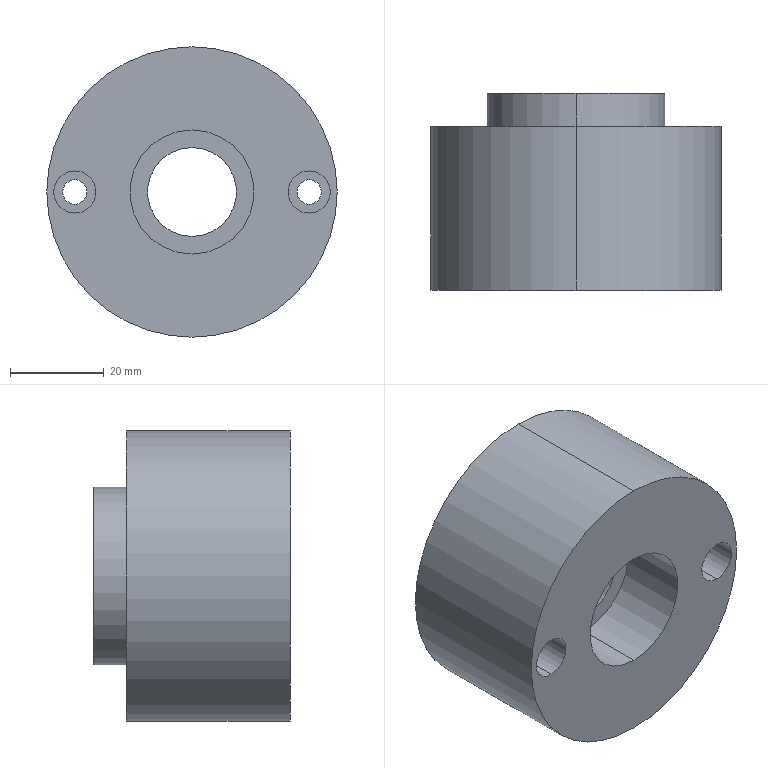Part | 1 solid | 24 faces | box 62 x 42 x 62 mm | volume 87250 mm3 | cylinder 16 | plane 6 | cone 2 | commonest cylinder face diameters 5.2 x4 9 x4 19 x2 26.5 x2 38 x2 62 x2
STEP:
#1=CARTESIAN_POINT('',(0.,20.,9.5));
#2=VERTEX_POINT('',#1);
#3=CARTESIAN_POINT('',(0.,20.,-9.5));
#4=VERTEX_POINT('',#3);
#5=CARTESIAN_POINT('',(0.,20.,0.));
#6=DIRECTION('',(0.,-1.,0.));
#7=DIRECTION('',(0.,0.,-1.));
#8=AXIS2_PLACEMENT_3D('',#5,#6,#7);
#9=CIRCLE('',#8,9.5);
#10=EDGE_CURVE('',#2,#4,#9,.T.);
#11=ORIENTED_EDGE('',*,*,#10,.T.);
#12=CARTESIAN_POINT('',(0.,42.,-18.));
#13=VERTEX_POINT('',#12);
#14=CARTESIAN_POINT('',(0.,20.,-9.5));
#15=DIRECTION('',(0.,0.9328,-0.3604));
#16=VECTOR('',#15,1000.);
#17=LINE('',#14,#16);
#18=EDGE_CURVE('',#4,#13,#17,.T.);
#19=ORIENTED_EDGE('',*,*,#18,.T.);
#20=CARTESIAN_POINT('',(0.,42.,18.));
#21=VERTEX_POINT('',#20);
#22=CARTESIAN_POINT('',(0.,42.,0.));
#23=DIRECTION('',(0.,-1.,0.));
#24=DIRECTION('',(0.,0.,-1.));
#25=AXIS2_PLACEMENT_3D('',#22,#23,#24);
#26=CIRCLE('',#25,18.);
#27=EDGE_CURVE('',#21,#13,#26,.T.);
#28=ORIENTED_EDGE('',*,*,#27,.F.);
#29=CARTESIAN_POINT('',(0.,20.,9.5));
#30=DIRECTION('',(0.,0.9328,0.3604));
#31=VECTOR('',#30,1000.);
#32=LINE('',#29,#31);
#33=EDGE_CURVE('',#2,#21,#32,.T.);
#34=ORIENTED_EDGE('',*,*,#33,.F.);
#35=EDGE_LOOP('',(#11,#19,#28,#34));
#36=FACE_OUTER_BOUND('',#35,.T.);
#37=CARTESIAN_POINT('',(0.,20.,0.));
#38=DIRECTION('',(0.,1.,0.));
#39=DIRECTION('',(0.,0.,1.));
#40=AXIS2_PLACEMENT_3D('',#37,#38,#39);
#41=CONICAL_SURFACE('',#40,9.5,0.3687);
#42=ADVANCED_FACE('',(#36),#41,.F.);
#43=ORIENTED_EDGE('',*,*,#10,.F.);
#44=CARTESIAN_POINT('',(0.,15.,9.5));
#45=VERTEX_POINT('',#44);
#46=CARTESIAN_POINT('',(0.,15.,9.5));
#47=DIRECTION('',(0.,-1.,0.));
#48=VECTOR('',#47,1000.);
#49=LINE('',#46,#48);
#50=EDGE_CURVE('',#2,#45,#49,.T.);
#51=ORIENTED_EDGE('',*,*,#50,.T.);
#52=CARTESIAN_POINT('',(0.,15.,-9.5));
#53=VERTEX_POINT('',#52);
#54=CARTESIAN_POINT('',(0.,15.,0.));
#55=DIRECTION('',(0.,-1.,0.));
#56=DIRECTION('',(0.,0.,-1.));
#57=AXIS2_PLACEMENT_3D('',#54,#55,#56);
#58=CIRCLE('',#57,9.5);
#59=EDGE_CURVE('',#45,#53,#58,.T.);
#60=ORIENTED_EDGE('',*,*,#59,.T.);
#61=CARTESIAN_POINT('',(0.,15.,-9.5));
#62=DIRECTION('',(0.,-1.,0.));
#63=VECTOR('',#62,1000.);
#64=LINE('',#61,#63);
#65=EDGE_CURVE('',#4,#53,#64,.T.);
#66=ORIENTED_EDGE('',*,*,#65,.F.);
#67=EDGE_LOOP('',(#43,#51,#60,#66));
#68=FACE_OUTER_BOUND('',#67,.T.);
#69=CARTESIAN_POINT('',(0.,15.,0.));
#70=DIRECTION('',(0.,-1.,0.));
#71=DIRECTION('',(0.,0.,-1.));
#72=AXIS2_PLACEMENT_3D('',#69,#70,#71);
#73=CYLINDRICAL_SURFACE('',#72,9.5);
#74=ADVANCED_FACE('',(#68),#73,.F.);
#75=CARTESIAN_POINT('',(0.,15.,13.25));
#76=VERTEX_POINT('',#75);
#77=CARTESIAN_POINT('',(0.,15.,-13.25));
#78=VERTEX_POINT('',#77);
#79=CARTESIAN_POINT('',(0.,15.,0.));
#80=DIRECTION('',(0.,-1.,0.));
#81=DIRECTION('',(0.,0.,-1.));
#82=AXIS2_PLACEMENT_3D('',#79,#80,#81);
#83=CIRCLE('',#82,13.25);
#84=EDGE_CURVE('',#76,#78,#83,.T.);
#85=ORIENTED_EDGE('',*,*,#84,.F.);
#86=CARTESIAN_POINT('',(0.,0.,13.25));
#87=VERTEX_POINT('',#86);
#88=CARTESIAN_POINT('',(0.,0.,13.25));
#89=DIRECTION('',(0.,-1.,0.));
#90=VECTOR('',#89,1000.);
#91=LINE('',#88,#90);
#92=EDGE_CURVE('',#76,#87,#91,.T.);
#93=ORIENTED_EDGE('',*,*,#92,.T.);
#94=CARTESIAN_POINT('',(0.,0.,-13.25));
#95=VERTEX_POINT('',#94);
#96=CARTESIAN_POINT('',(0.,0.,0.));
#97=DIRECTION('',(0.,-1.,0.));
#98=DIRECTION('',(0.,0.,-1.));
#99=AXIS2_PLACEMENT_3D('',#96,#97,#98);
#100=CIRCLE('',#99,13.25);
#101=EDGE_CURVE('',#87,#95,#100,.T.);
#102=ORIENTED_EDGE('',*,*,#101,.T.);
#103=CARTESIAN_POINT('',(0.,0.,-13.25));
#104=DIRECTION('',(0.,-1.,0.));
#105=VECTOR('',#104,1000.);
#106=LINE('',#103,#105);
#107=EDGE_CURVE('',#78,#95,#106,.T.);
#108=ORIENTED_EDGE('',*,*,#107,.F.);
#109=EDGE_LOOP('',(#85,#93,#102,#108));
#110=FACE_OUTER_BOUND('',#109,.T.);
#111=CARTESIAN_POINT('',(0.,0.,0.));
#112=DIRECTION('',(0.,-1.,0.));
#113=DIRECTION('',(0.,0.,-1.));
#114=AXIS2_PLACEMENT_3D('',#111,#112,#113);
#115=CYLINDRICAL_SURFACE('',#114,13.25);
#116=ADVANCED_FACE('',(#110),#115,.F.);
#117=CARTESIAN_POINT('',(-25.,35.,-2.6));
#118=VERTEX_POINT('',#117);
#119=CARTESIAN_POINT('',(-25.,35.,2.6));
#120=VERTEX_POINT('',#119);
#121=CARTESIAN_POINT('',(-25.,35.,0.));
#122=DIRECTION('',(0.,1.,0.));
#123=DIRECTION('',(0.,0.,1.));
#124=AXIS2_PLACEMENT_3D('',#121,#122,#123);
#125=CIRCLE('',#124,2.6);
#126=EDGE_CURVE('',#118,#120,#125,.T.);
#127=ORIENTED_EDGE('',*,*,#126,.T.);
#128=CARTESIAN_POINT('',(-25.,20.,2.6));
#129=VERTEX_POINT('',#128);
#130=CARTESIAN_POINT('',(-25.,42.,2.6));
#131=DIRECTION('',(0.,-1.,0.));
#132=VECTOR('',#131,1000.);
#133=LINE('',#130,#132);
#134=EDGE_CURVE('',#120,#129,#133,.T.);
#135=ORIENTED_EDGE('',*,*,#134,.T.);
#136=CARTESIAN_POINT('',(-25.,20.,-2.6));
#137=VERTEX_POINT('',#136);
#138=CARTESIAN_POINT('',(-25.,20.,0.));
#139=DIRECTION('',(0.,-1.,0.));
#140=DIRECTION('',(0.,0.,-1.));
#141=AXIS2_PLACEMENT_3D('',#138,#139,#140);
#142=CIRCLE('',#141,2.6);
#143=EDGE_CURVE('',#129,#137,#142,.T.);
#144=ORIENTED_EDGE('',*,*,#143,.T.);
#145=CARTESIAN_POINT('',(-25.,42.,-2.6));
#146=DIRECTION('',(0.,-1.,0.));
#147=VECTOR('',#146,1000.);
#148=LINE('',#145,#147);
#149=EDGE_CURVE('',#118,#137,#148,.T.);
#150=ORIENTED_EDGE('',*,*,#149,.F.);
#151=EDGE_LOOP('',(#127,#135,#144,#150));
#152=FACE_OUTER_BOUND('',#151,.T.);
#153=CARTESIAN_POINT('',(-25.,42.,0.));
#154=DIRECTION('',(0.,-1.,0.));
#155=DIRECTION('',(0.,0.,-1.));
#156=AXIS2_PLACEMENT_3D('',#153,#154,#155);
#157=CYLINDRICAL_SURFACE('',#156,2.6);
#158=ADVANCED_FACE('',(#152),#157,.F.);
#159=CARTESIAN_POINT('',(25.,35.,-2.6));
#160=VERTEX_POINT('',#159);
#161=CARTESIAN_POINT('',(25.,35.,2.6));
#162=VERTEX_POINT('',#161);
#163=CARTESIAN_POINT('',(25.,35.,0.));
#164=DIRECTION('',(0.,1.,0.));
#165=DIRECTION('',(0.,0.,1.));
#166=AXIS2_PLACEMENT_3D('',#163,#164,#165);
#167=CIRCLE('',#166,2.6);
#168=EDGE_CURVE('',#160,#162,#167,.T.);
#169=ORIENTED_EDGE('',*,*,#168,.T.);
#170=CARTESIAN_POINT('',(25.,20.,2.6));
#171=VERTEX_POINT('',#170);
#172=CARTESIAN_POINT('',(25.,42.,2.6));
#173=DIRECTION('',(0.,-1.,0.));
#174=VECTOR('',#173,1000.);
#175=LINE('',#172,#174);
#176=EDGE_CURVE('',#162,#171,#175,.T.);
#177=ORIENTED_EDGE('',*,*,#176,.T.);
#178=CARTESIAN_POINT('',(25.,20.,-2.6));
#179=VERTEX_POINT('',#178);
#180=CARTESIAN_POINT('',(25.,20.,0.));
#181=DIRECTION('',(0.,-1.,0.));
#182=DIRECTION('',(0.,0.,1.));
#183=AXIS2_PLACEMENT_3D('',#180,#181,#182);
#184=CIRCLE('',#183,2.6);
#185=EDGE_CURVE('',#171,#179,#184,.T.);
#186=ORIENTED_EDGE('',*,*,#185,.T.);
#187=CARTESIAN_POINT('',(25.,42.,-2.6));
#188=DIRECTION('',(0.,-1.,0.));
#189=VECTOR('',#188,1000.);
#190=LINE('',#187,#189);
#191=EDGE_CURVE('',#160,#179,#190,.T.);
#192=ORIENTED_EDGE('',*,*,#191,.F.);
#193=EDGE_LOOP('',(#169,#177,#186,#192));
#194=FACE_OUTER_BOUND('',#193,.T.);
#195=CARTESIAN_POINT('',(25.,42.,0.));
#196=DIRECTION('',(0.,-1.,0.));
#197=DIRECTION('',(0.,0.,-1.));
#198=AXIS2_PLACEMENT_3D('',#195,#196,#197);
#199=CYLINDRICAL_SURFACE('',#198,2.6);
#200=ADVANCED_FACE('',(#194),#199,.F.);
#201=CARTESIAN_POINT('',(-25.,20.,4.5));
#202=VERTEX_POINT('',#201);
#203=CARTESIAN_POINT('',(-25.,20.,-4.5));
#204=VERTEX_POINT('',#203);
#205=CARTESIAN_POINT('',(-25.,20.,0.));
#206=DIRECTION('',(0.,-1.,0.));
#207=DIRECTION('',(0.,0.,-1.));
#208=AXIS2_PLACEMENT_3D('',#205,#206,#207);
#209=CIRCLE('',#208,4.5);
#210=EDGE_CURVE('',#202,#204,#209,.T.);
#211=ORIENTED_EDGE('',*,*,#210,.F.);
#212=CARTESIAN_POINT('',(-25.,0.,4.5));
#213=VERTEX_POINT('',#212);
#214=CARTESIAN_POINT('',(-25.,20.,4.5));
#215=DIRECTION('',(0.,-1.,0.));
#216=VECTOR('',#215,1000.);
#217=LINE('',#214,#216);
#218=EDGE_CURVE('',#202,#213,#217,.T.);
#219=ORIENTED_EDGE('',*,*,#218,.T.);
#220=CARTESIAN_POINT('',(-25.,0.,-4.5));
#221=VERTEX_POINT('',#220);
#222=CARTESIAN_POINT('',(-25.,0.,0.));
#223=DIRECTION('',(0.,-1.,0.));
#224=DIRECTION('',(0.,0.,-1.));
#225=AXIS2_PLACEMENT_3D('',#222,#223,#224);
#226=CIRCLE('',#225,4.5);
#227=EDGE_CURVE('',#213,#221,#226,.T.);
#228=ORIENTED_EDGE('',*,*,#227,.T.);
#229=CARTESIAN_POINT('',(-25.,20.,-4.5));
#230=DIRECTION('',(0.,-1.,0.));
#231=VECTOR('',#230,1000.);
#232=LINE('',#229,#231);
#233=EDGE_CURVE('',#204,#221,#232,.T.);
#234=ORIENTED_EDGE('',*,*,#233,.F.);
#235=EDGE_LOOP('',(#211,#219,#228,#234));
#236=FACE_OUTER_BOUND('',#235,.T.);
#237=CARTESIAN_POINT('',(-25.,20.,0.));
#238=DIRECTION('',(0.,-1.,0.));
#239=DIRECTION('',(0.,0.,-1.));
#240=AXIS2_PLACEMENT_3D('',#237,#238,#239);
#241=CYLINDRICAL_SURFACE('',#240,4.5);
#242=ADVANCED_FACE('',(#236),#241,.F.);
#243=CARTESIAN_POINT('',(25.,20.,4.5));
#244=VERTEX_POINT('',#243);
#245=CARTESIAN_POINT('',(25.,20.,-4.5));
#246=VERTEX_POINT('',#245);
#247=CARTESIAN_POINT('',(25.,20.,0.));
#248=DIRECTION('',(0.,-1.,0.));
#249=DIRECTION('',(0.,0.,1.));
#250=AXIS2_PLACEMENT_3D('',#247,#248,#249);
#251=CIRCLE('',#250,4.5);
#252=EDGE_CURVE('',#244,#246,#251,.T.);
#253=ORIENTED_EDGE('',*,*,#252,.F.);
#254=CARTESIAN_POINT('',(25.,0.,4.5));
#255=VERTEX_POINT('',#254);
#256=CARTESIAN_POINT('',(25.,20.,4.5));
#257=DIRECTION('',(0.,-1.,0.));
#258=VECTOR('',#257,1000.);
#259=LINE('',#256,#258);
#260=EDGE_CURVE('',#244,#255,#259,.T.);
#261=ORIENTED_EDGE('',*,*,#260,.T.);
#262=CARTESIAN_POINT('',(25.,0.,-4.5));
#263=VERTEX_POINT('',#262);
#264=CARTESIAN_POINT('',(25.,0.,0.));
#265=DIRECTION('',(0.,-1.,0.));
#266=DIRECTION('',(0.,0.,1.));
#267=AXIS2_PLACEMENT_3D('',#264,#265,#266);
#268=CIRCLE('',#267,4.5);
#269=EDGE_CURVE('',#255,#263,#268,.T.);
#270=ORIENTED_EDGE('',*,*,#269,.T.);
#271=CARTESIAN_POINT('',(25.,20.,-4.5));
#272=DIRECTION('',(0.,-1.,0.));
#273=VECTOR('',#272,1000.);
#274=LINE('',#271,#273);
#275=EDGE_CURVE('',#246,#263,#274,.T.);
#276=ORIENTED_EDGE('',*,*,#275,.F.);
#277=EDGE_LOOP('',(#253,#261,#270,#276));
#278=FACE_OUTER_BOUND('',#277,.T.);
#279=CARTESIAN_POINT('',(25.,20.,0.));
#280=DIRECTION('',(0.,-1.,0.));
#281=DIRECTION('',(0.,0.,-1.));
#282=AXIS2_PLACEMENT_3D('',#279,#280,#281);
#283=CYLINDRICAL_SURFACE('',#282,4.5);
#284=ADVANCED_FACE('',(#278),#283,.F.);
#285=CARTESIAN_POINT('',(0.,42.,19.));
#286=VERTEX_POINT('',#285);
#287=CARTESIAN_POINT('',(0.,42.,-19.));
#288=VERTEX_POINT('',#287);
#289=CARTESIAN_POINT('',(0.,42.,0.));
#290=DIRECTION('',(0.,1.,0.));
#291=DIRECTION('',(0.,0.,1.));
#292=AXIS2_PLACEMENT_3D('',#289,#290,#291);
#293=CIRCLE('',#292,19.);
#294=EDGE_CURVE('',#286,#288,#293,.T.);
#295=ORIENTED_EDGE('',*,*,#294,.F.);
#296=CARTESIAN_POINT('',(0.,35.,19.));
#297=VERTEX_POINT('',#296);
#298=CARTESIAN_POINT('',(0.,42.,19.));
#299=DIRECTION('',(0.,-1.,0.));
#300=VECTOR('',#299,1000.);
#301=LINE('',#298,#300);
#302=EDGE_CURVE('',#286,#297,#301,.T.);
#303=ORIENTED_EDGE('',*,*,#302,.T.);
#304=CARTESIAN_POINT('',(0.,35.,-19.));
#305=VERTEX_POINT('',#304);
#306=CARTESIAN_POINT('',(0.,35.,0.));
#307=DIRECTION('',(0.,1.,0.));
#308=DIRECTION('',(0.,0.,1.));
#309=AXIS2_PLACEMENT_3D('',#306,#307,#308);
#310=CIRCLE('',#309,19.);
#311=EDGE_CURVE('',#297,#305,#310,.T.);
#312=ORIENTED_EDGE('',*,*,#311,.T.);
#313=CARTESIAN_POINT('',(0.,42.,-19.));
#314=DIRECTION('',(0.,-1.,0.));
#315=VECTOR('',#314,1000.);
#316=LINE('',#313,#315);
#317=EDGE_CURVE('',#288,#305,#316,.T.);
#318=ORIENTED_EDGE('',*,*,#317,.F.);
#319=EDGE_LOOP('',(#295,#303,#312,#318));
#320=FACE_OUTER_BOUND('',#319,.T.);
#321=CARTESIAN_POINT('',(0.,42.,0.));
#322=DIRECTION('',(0.,-1.,0.));
#323=DIRECTION('',(0.,0.,-1.));
#324=AXIS2_PLACEMENT_3D('',#321,#322,#323);
#325=CYLINDRICAL_SURFACE('',#324,19.);
#326=ADVANCED_FACE('',(#320),#325,.T.);
#327=CARTESIAN_POINT('',(0.,35.,31.));
#328=VERTEX_POINT('',#327);
#329=CARTESIAN_POINT('',(0.,35.,-31.));
#330=VERTEX_POINT('',#329);
#331=CARTESIAN_POINT('',(0.,35.,0.));
#332=DIRECTION('',(0.,1.,0.));
#333=DIRECTION('',(0.,0.,1.));
#334=AXIS2_PLACEMENT_3D('',#331,#332,#333);
#335=CIRCLE('',#334,31.);
#336=EDGE_CURVE('',#328,#330,#335,.T.);
#337=ORIENTED_EDGE('',*,*,#336,.F.);
#338=CARTESIAN_POINT('',(0.,0.,31.));
#339=VERTEX_POINT('',#338);
#340=CARTESIAN_POINT('',(0.,35.,31.));
#341=DIRECTION('',(0.,-1.,0.));
#342=VECTOR('',#341,1000.);
#343=LINE('',#340,#342);
#344=EDGE_CURVE('',#328,#339,#343,.T.);
#345=ORIENTED_EDGE('',*,*,#344,.T.);
#346=CARTESIAN_POINT('',(0.,0.,-31.));
#347=VERTEX_POINT('',#346);
#348=CARTESIAN_POINT('',(0.,0.,0.));
#349=DIRECTION('',(0.,1.,0.));
#350=DIRECTION('',(0.,0.,1.));
#351=AXIS2_PLACEMENT_3D('',#348,#349,#350);
#352=CIRCLE('',#351,31.);
#353=EDGE_CURVE('',#339,#347,#352,.T.);
#354=ORIENTED_EDGE('',*,*,#353,.T.);
#355=CARTESIAN_POINT('',(0.,35.,-31.));
#356=DIRECTION('',(0.,-1.,0.));
#357=VECTOR('',#356,1000.);
#358=LINE('',#355,#357);
#359=EDGE_CURVE('',#330,#347,#358,.T.);
#360=ORIENTED_EDGE('',*,*,#359,.F.);
#361=EDGE_LOOP('',(#337,#345,#354,#360));
#362=FACE_OUTER_BOUND('',#361,.T.);
#363=CARTESIAN_POINT('',(0.,35.,0.));
#364=DIRECTION('',(0.,-1.,0.));
#365=DIRECTION('',(0.,0.,-1.));
#366=AXIS2_PLACEMENT_3D('',#363,#364,#365);
#367=CYLINDRICAL_SURFACE('',#366,31.);
#368=ADVANCED_FACE('',(#362),#367,.T.);
#369=ORIENTED_EDGE('',*,*,#344,.F.);
#370=CARTESIAN_POINT('',(0.,35.,0.));
#371=DIRECTION('',(0.,1.,0.));
#372=DIRECTION('',(0.,0.,1.));
#373=AXIS2_PLACEMENT_3D('',#370,#371,#372);
#374=CIRCLE('',#373,31.);
#375=EDGE_CURVE('',#330,#328,#374,.T.);
#376=ORIENTED_EDGE('',*,*,#375,.F.);
#377=ORIENTED_EDGE('',*,*,#359,.T.);
#378=CARTESIAN_POINT('',(0.,0.,0.));
#379=DIRECTION('',(0.,1.,0.));
#380=DIRECTION('',(0.,0.,1.));
#381=AXIS2_PLACEMENT_3D('',#378,#379,#380);
#382=CIRCLE('',#381,31.);
#383=EDGE_CURVE('',#347,#339,#382,.T.);
#384=ORIENTED_EDGE('',*,*,#383,.T.);
#385=EDGE_LOOP('',(#369,#376,#377,#384));
#386=FACE_OUTER_BOUND('',#385,.T.);
#387=CARTESIAN_POINT('',(0.,35.,0.));
#388=DIRECTION('',(0.,-1.,0.));
#389=DIRECTION('',(0.,0.,-1.));
#390=AXIS2_PLACEMENT_3D('',#387,#388,#389);
#391=CYLINDRICAL_SURFACE('',#390,31.);
#392=ADVANCED_FACE('',(#386),#391,.T.);
#393=ORIENTED_EDGE('',*,*,#126,.F.);
#394=CARTESIAN_POINT('',(-25.,35.,0.));
#395=DIRECTION('',(0.,1.,0.));
#396=DIRECTION('',(0.,0.,1.));
#397=AXIS2_PLACEMENT_3D('',#394,#395,#396);
#398=CIRCLE('',#397,2.6);
#399=EDGE_CURVE('',#120,#118,#398,.T.);
#400=ORIENTED_EDGE('',*,*,#399,.F.);
#401=EDGE_LOOP('',(#393,#400));
#402=FACE_BOUND('',#401,.T.);
#403=ORIENTED_EDGE('',*,*,#168,.F.);
#404=CARTESIAN_POINT('',(25.,35.,0.));
#405=DIRECTION('',(0.,1.,0.));
#406=DIRECTION('',(0.,0.,1.));
#407=AXIS2_PLACEMENT_3D('',#404,#405,#406);
#408=CIRCLE('',#407,2.6);
#409=EDGE_CURVE('',#162,#160,#408,.T.);
#410=ORIENTED_EDGE('',*,*,#409,.F.);
#411=EDGE_LOOP('',(#403,#410));
#412=FACE_BOUND('',#411,.T.);
#413=CARTESIAN_POINT('',(0.,35.,0.));
#414=DIRECTION('',(0.,1.,0.));
#415=DIRECTION('',(0.,0.,1.));
#416=AXIS2_PLACEMENT_3D('',#413,#414,#415);
#417=CIRCLE('',#416,19.);
#418=EDGE_CURVE('',#305,#297,#417,.T.);
#419=ORIENTED_EDGE('',*,*,#418,.F.);
#420=ORIENTED_EDGE('',*,*,#311,.F.);
#421=EDGE_LOOP('',(#419,#420));
#422=FACE_BOUND('',#421,.T.);
#423=ORIENTED_EDGE('',*,*,#375,.T.);
#424=ORIENTED_EDGE('',*,*,#336,.T.);
#425=EDGE_LOOP('',(#423,#424));
#426=FACE_OUTER_BOUND('',#425,.T.);
#427=CARTESIAN_POINT('',(0.,35.,0.));
#428=DIRECTION('',(0.,1.,0.));
#429=DIRECTION('',(0.,0.,1.));
#430=AXIS2_PLACEMENT_3D('',#427,#428,#429);
#431=PLANE('',#430);
#432=ADVANCED_FACE('',(#402,#412,#422,#426),#431,.T.);
#433=CARTESIAN_POINT('',(0.,0.,0.));
#434=DIRECTION('',(0.,-1.,0.));
#435=DIRECTION('',(0.,0.,-1.));
#436=AXIS2_PLACEMENT_3D('',#433,#434,#435);
#437=CIRCLE('',#436,13.25);
#438=EDGE_CURVE('',#95,#87,#437,.T.);
#439=ORIENTED_EDGE('',*,*,#438,.F.);
#440=ORIENTED_EDGE('',*,*,#101,.F.);
#441=EDGE_LOOP('',(#439,#440));
#442=FACE_BOUND('',#441,.T.);
#443=CARTESIAN_POINT('',(-25.,0.,0.));
#444=DIRECTION('',(0.,-1.,0.));
#445=DIRECTION('',(0.,0.,-1.));
#446=AXIS2_PLACEMENT_3D('',#443,#444,#445);
#447=CIRCLE('',#446,4.5);
#448=EDGE_CURVE('',#221,#213,#447,.T.);
#449=ORIENTED_EDGE('',*,*,#448,.F.);
#450=ORIENTED_EDGE('',*,*,#227,.F.);
#451=EDGE_LOOP('',(#449,#450));
#452=FACE_BOUND('',#451,.T.);
#453=CARTESIAN_POINT('',(25.,0.,0.));
#454=DIRECTION('',(0.,-1.,0.));
#455=DIRECTION('',(0.,0.,1.));
#456=AXIS2_PLACEMENT_3D('',#453,#454,#455);
#457=CIRCLE('',#456,4.5);
#458=EDGE_CURVE('',#263,#255,#457,.T.);
#459=ORIENTED_EDGE('',*,*,#458,.F.);
#460=ORIENTED_EDGE('',*,*,#269,.F.);
#461=EDGE_LOOP('',(#459,#460));
#462=FACE_BOUND('',#461,.T.);
#463=ORIENTED_EDGE('',*,*,#383,.F.);
#464=ORIENTED_EDGE('',*,*,#353,.F.);
#465=EDGE_LOOP('',(#463,#464));
#466=FACE_OUTER_BOUND('',#465,.T.);
#467=CARTESIAN_POINT('',(0.,0.,0.));
#468=DIRECTION('',(0.,1.,0.));
#469=DIRECTION('',(0.,0.,1.));
#470=AXIS2_PLACEMENT_3D('',#467,#468,#469);
#471=PLANE('',#470);
#472=ADVANCED_FACE('',(#442,#452,#462,#466),#471,.F.);
#473=ORIENTED_EDGE('',*,*,#302,.F.);
#474=CARTESIAN_POINT('',(0.,42.,0.));
#475=DIRECTION('',(0.,1.,0.));
#476=DIRECTION('',(0.,0.,1.));
#477=AXIS2_PLACEMENT_3D('',#474,#475,#476);
#478=CIRCLE('',#477,19.);
#479=EDGE_CURVE('',#288,#286,#478,.T.);
#480=ORIENTED_EDGE('',*,*,#479,.F.);
#481=ORIENTED_EDGE('',*,*,#317,.T.);
#482=ORIENTED_EDGE('',*,*,#418,.T.);
#483=EDGE_LOOP('',(#473,#480,#481,#482));
#484=FACE_OUTER_BOUND('',#483,.T.);
#485=CARTESIAN_POINT('',(0.,42.,0.));
#486=DIRECTION('',(0.,-1.,0.));
#487=DIRECTION('',(0.,0.,-1.));
#488=AXIS2_PLACEMENT_3D('',#485,#486,#487);
#489=CYLINDRICAL_SURFACE('',#488,19.);
#490=ADVANCED_FACE('',(#484),#489,.T.);
#491=ORIENTED_EDGE('',*,*,#27,.T.);
#492=CARTESIAN_POINT('',(0.,42.,0.));
#493=DIRECTION('',(0.,-1.,0.));
#494=DIRECTION('',(0.,0.,-1.));
#495=AXIS2_PLACEMENT_3D('',#492,#493,#494);
#496=CIRCLE('',#495,18.);
#497=EDGE_CURVE('',#13,#21,#496,.T.);
#498=ORIENTED_EDGE('',*,*,#497,.T.);
#499=EDGE_LOOP('',(#491,#498));
#500=FACE_BOUND('',#499,.T.);
#501=ORIENTED_EDGE('',*,*,#479,.T.);
#502=ORIENTED_EDGE('',*,*,#294,.T.);
#503=EDGE_LOOP('',(#501,#502));
#504=FACE_OUTER_BOUND('',#503,.T.);
#505=CARTESIAN_POINT('',(0.,42.,0.));
#506=DIRECTION('',(0.,1.,0.));
#507=DIRECTION('',(0.,0.,1.));
#508=AXIS2_PLACEMENT_3D('',#505,#506,#507);
#509=PLANE('',#508);
#510=ADVANCED_FACE('',(#500,#504),#509,.T.);
#511=ORIENTED_EDGE('',*,*,#260,.F.);
#512=CARTESIAN_POINT('',(25.,20.,0.));
#513=DIRECTION('',(0.,-1.,0.));
#514=DIRECTION('',(0.,0.,1.));
#515=AXIS2_PLACEMENT_3D('',#512,#513,#514);
#516=CIRCLE('',#515,4.5);
#517=EDGE_CURVE('',#246,#244,#516,.T.);
#518=ORIENTED_EDGE('',*,*,#517,.F.);
#519=ORIENTED_EDGE('',*,*,#275,.T.);
#520=ORIENTED_EDGE('',*,*,#458,.T.);
#521=EDGE_LOOP('',(#511,#518,#519,#520));
#522=FACE_OUTER_BOUND('',#521,.T.);
#523=CARTESIAN_POINT('',(25.,20.,0.));
#524=DIRECTION('',(0.,-1.,0.));
#525=DIRECTION('',(0.,0.,-1.));
#526=AXIS2_PLACEMENT_3D('',#523,#524,#525);
#527=CYLINDRICAL_SURFACE('',#526,4.5);
#528=ADVANCED_FACE('',(#522),#527,.F.);
#529=CARTESIAN_POINT('',(25.,20.,0.));
#530=DIRECTION('',(0.,-1.,0.));
#531=DIRECTION('',(0.,0.,1.));
#532=AXIS2_PLACEMENT_3D('',#529,#530,#531);
#533=CIRCLE('',#532,2.6);
#534=EDGE_CURVE('',#179,#171,#533,.T.);
#535=ORIENTED_EDGE('',*,*,#534,.F.);
#536=ORIENTED_EDGE('',*,*,#185,.F.);
#537=EDGE_LOOP('',(#535,#536));
#538=FACE_BOUND('',#537,.T.);
#539=ORIENTED_EDGE('',*,*,#517,.T.);
#540=ORIENTED_EDGE('',*,*,#252,.T.);
#541=EDGE_LOOP('',(#539,#540));
#542=FACE_OUTER_BOUND('',#541,.T.);
#543=CARTESIAN_POINT('',(25.,20.,0.));
#544=DIRECTION('',(0.,1.,0.));
#545=DIRECTION('',(0.,0.,1.));
#546=AXIS2_PLACEMENT_3D('',#543,#544,#545);
#547=PLANE('',#546);
#548=ADVANCED_FACE('',(#538,#542),#547,.F.);
#549=ORIENTED_EDGE('',*,*,#218,.F.);
#550=CARTESIAN_POINT('',(-25.,20.,0.));
#551=DIRECTION('',(0.,-1.,0.));
#552=DIRECTION('',(0.,0.,-1.));
#553=AXIS2_PLACEMENT_3D('',#550,#551,#552);
#554=CIRCLE('',#553,4.5);
#555=EDGE_CURVE('',#204,#202,#554,.T.);
#556=ORIENTED_EDGE('',*,*,#555,.F.);
#557=ORIENTED_EDGE('',*,*,#233,.T.);
#558=ORIENTED_EDGE('',*,*,#448,.T.);
#559=EDGE_LOOP('',(#549,#556,#557,#558));
#560=FACE_OUTER_BOUND('',#559,.T.);
#561=CARTESIAN_POINT('',(-25.,20.,0.));
#562=DIRECTION('',(0.,-1.,0.));
#563=DIRECTION('',(0.,0.,-1.));
#564=AXIS2_PLACEMENT_3D('',#561,#562,#563);
#565=CYLINDRICAL_SURFACE('',#564,4.5);
#566=ADVANCED_FACE('',(#560),#565,.F.);
#567=CARTESIAN_POINT('',(-25.,20.,0.));
#568=DIRECTION('',(0.,-1.,0.));
#569=DIRECTION('',(0.,0.,-1.));
#570=AXIS2_PLACEMENT_3D('',#567,#568,#569);
#571=CIRCLE('',#570,2.6);
#572=EDGE_CURVE('',#137,#129,#571,.T.);
#573=ORIENTED_EDGE('',*,*,#572,.F.);
#574=ORIENTED_EDGE('',*,*,#143,.F.);
#575=EDGE_LOOP('',(#573,#574));
#576=FACE_BOUND('',#575,.T.);
#577=ORIENTED_EDGE('',*,*,#555,.T.);
#578=ORIENTED_EDGE('',*,*,#210,.T.);
#579=EDGE_LOOP('',(#577,#578));
#580=FACE_OUTER_BOUND('',#579,.T.);
#581=CARTESIAN_POINT('',(-25.,20.,0.));
#582=DIRECTION('',(0.,-1.,0.));
#583=DIRECTION('',(0.,0.,-1.));
#584=AXIS2_PLACEMENT_3D('',#581,#582,#583);
#585=PLANE('',#584);
#586=ADVANCED_FACE('',(#576,#580),#585,.T.);
#587=ORIENTED_EDGE('',*,*,#176,.F.);
#588=ORIENTED_EDGE('',*,*,#409,.T.);
#589=ORIENTED_EDGE('',*,*,#191,.T.);
#590=ORIENTED_EDGE('',*,*,#534,.T.);
#591=EDGE_LOOP('',(#587,#588,#589,#590));
#592=FACE_OUTER_BOUND('',#591,.T.);
#593=CARTESIAN_POINT('',(25.,42.,0.));
#594=DIRECTION('',(0.,-1.,0.));
#595=DIRECTION('',(0.,0.,-1.));
#596=AXIS2_PLACEMENT_3D('',#593,#594,#595);
#597=CYLINDRICAL_SURFACE('',#596,2.6);
#598=ADVANCED_FACE('',(#592),#597,.F.);
#599=ORIENTED_EDGE('',*,*,#134,.F.);
#600=ORIENTED_EDGE('',*,*,#399,.T.);
#601=ORIENTED_EDGE('',*,*,#149,.T.);
#602=ORIENTED_EDGE('',*,*,#572,.T.);
#603=EDGE_LOOP('',(#599,#600,#601,#602));
#604=FACE_OUTER_BOUND('',#603,.T.);
#605=CARTESIAN_POINT('',(-25.,42.,0.));
#606=DIRECTION('',(0.,-1.,0.));
#607=DIRECTION('',(0.,0.,-1.));
#608=AXIS2_PLACEMENT_3D('',#605,#606,#607);
#609=CYLINDRICAL_SURFACE('',#608,2.6);
#610=ADVANCED_FACE('',(#604),#609,.F.);
#611=CARTESIAN_POINT('',(0.,15.,0.));
#612=DIRECTION('',(0.,-1.,0.));
#613=DIRECTION('',(0.,0.,-1.));
#614=AXIS2_PLACEMENT_3D('',#611,#612,#613);
#615=CIRCLE('',#614,9.5);
#616=EDGE_CURVE('',#53,#45,#615,.T.);
#617=ORIENTED_EDGE('',*,*,#616,.F.);
#618=ORIENTED_EDGE('',*,*,#59,.F.);
#619=EDGE_LOOP('',(#617,#618));
#620=FACE_BOUND('',#619,.T.);
#621=CARTESIAN_POINT('',(0.,15.,0.));
#622=DIRECTION('',(0.,-1.,0.));
#623=DIRECTION('',(0.,0.,-1.));
#624=AXIS2_PLACEMENT_3D('',#621,#622,#623);
#625=CIRCLE('',#624,13.25);
#626=EDGE_CURVE('',#78,#76,#625,.T.);
#627=ORIENTED_EDGE('',*,*,#626,.T.);
#628=ORIENTED_EDGE('',*,*,#84,.T.);
#629=EDGE_LOOP('',(#627,#628));
#630=FACE_OUTER_BOUND('',#629,.T.);
#631=CARTESIAN_POINT('',(0.,15.,0.));
#632=DIRECTION('',(0.,1.,0.));
#633=DIRECTION('',(0.,0.,1.));
#634=AXIS2_PLACEMENT_3D('',#631,#632,#633);
#635=PLANE('',#634);
#636=ADVANCED_FACE('',(#620,#630),#635,.F.);
#637=ORIENTED_EDGE('',*,*,#92,.F.);
#638=ORIENTED_EDGE('',*,*,#626,.F.);
#639=ORIENTED_EDGE('',*,*,#107,.T.);
#640=ORIENTED_EDGE('',*,*,#438,.T.);
#641=EDGE_LOOP('',(#637,#638,#639,#640));
#642=FACE_OUTER_BOUND('',#641,.T.);
#643=CARTESIAN_POINT('',(0.,0.,0.));
#644=DIRECTION('',(0.,-1.,0.));
#645=DIRECTION('',(0.,0.,-1.));
#646=AXIS2_PLACEMENT_3D('',#643,#644,#645);
#647=CYLINDRICAL_SURFACE('',#646,13.25);
#648=ADVANCED_FACE('',(#642),#647,.F.);
#649=ORIENTED_EDGE('',*,*,#50,.F.);
#650=CARTESIAN_POINT('',(0.,20.,0.));
#651=DIRECTION('',(0.,-1.,0.));
#652=DIRECTION('',(0.,0.,-1.));
#653=AXIS2_PLACEMENT_3D('',#650,#651,#652);
#654=CIRCLE('',#653,9.5);
#655=EDGE_CURVE('',#4,#2,#654,.T.);
#656=ORIENTED_EDGE('',*,*,#655,.F.);
#657=ORIENTED_EDGE('',*,*,#65,.T.);
#658=ORIENTED_EDGE('',*,*,#616,.T.);
#659=EDGE_LOOP('',(#649,#656,#657,#658));
#660=FACE_OUTER_BOUND('',#659,.T.);
#661=CARTESIAN_POINT('',(0.,15.,0.));
#662=DIRECTION('',(0.,-1.,0.));
#663=DIRECTION('',(0.,0.,-1.));
#664=AXIS2_PLACEMENT_3D('',#661,#662,#663);
#665=CYLINDRICAL_SURFACE('',#664,9.5);
#666=ADVANCED_FACE('',(#660),#665,.F.);
#667=ORIENTED_EDGE('',*,*,#18,.F.);
#668=ORIENTED_EDGE('',*,*,#655,.T.);
#669=ORIENTED_EDGE('',*,*,#33,.T.);
#670=ORIENTED_EDGE('',*,*,#497,.F.);
#671=EDGE_LOOP('',(#667,#668,#669,#670));
#672=FACE_OUTER_BOUND('',#671,.T.);
#673=CARTESIAN_POINT('',(0.,20.,0.));
#674=DIRECTION('',(0.,1.,0.));
#675=DIRECTION('',(0.,0.,1.));
#676=AXIS2_PLACEMENT_3D('',#673,#674,#675);
#677=CONICAL_SURFACE('',#676,9.5,0.3687);
#678=ADVANCED_FACE('',(#672),#677,.F.);
#679=CLOSED_SHELL('',(#42,#74,#116,#158,#200,#242,#284,#326,#368,#392,#432,#472,#490,#510,#528,#548,#566,#586,#598,#610,#636,#648,#666,#678));
#680=MANIFOLD_SOLID_BREP('',#679);
#681=CARTESIAN_POINT('',(0.,0.,0.));
#682=DIRECTION('',(0.,0.,1.));
#683=DIRECTION('',(1.,0.,0.));
#684=AXIS2_PLACEMENT_3D('',#681,#682,#683);
#685=(LENGTH_UNIT()NAMED_UNIT(*)SI_UNIT(.MILLI.,.METRE.));
#686=UNCERTAINTY_MEASURE_WITH_UNIT(LENGTH_MEASURE(0.00001),#685,'','');
#687=(NAMED_UNIT(*)PLANE_ANGLE_UNIT()SI_UNIT($,.RADIAN.));
#688=(NAMED_UNIT(*)SI_UNIT($,.STERADIAN.)SOLID_ANGLE_UNIT());
#689=(GEOMETRIC_REPRESENTATION_CONTEXT(3)GLOBAL_UNCERTAINTY_ASSIGNED_CONTEXT((#686))GLOBAL_UNIT_ASSIGNED_CONTEXT((#685,#687,#688))REPRESENTATION_CONTEXT('',''));
#690=ADVANCED_BREP_SHAPE_REPRESENTATION('',(#680,#684),#689);